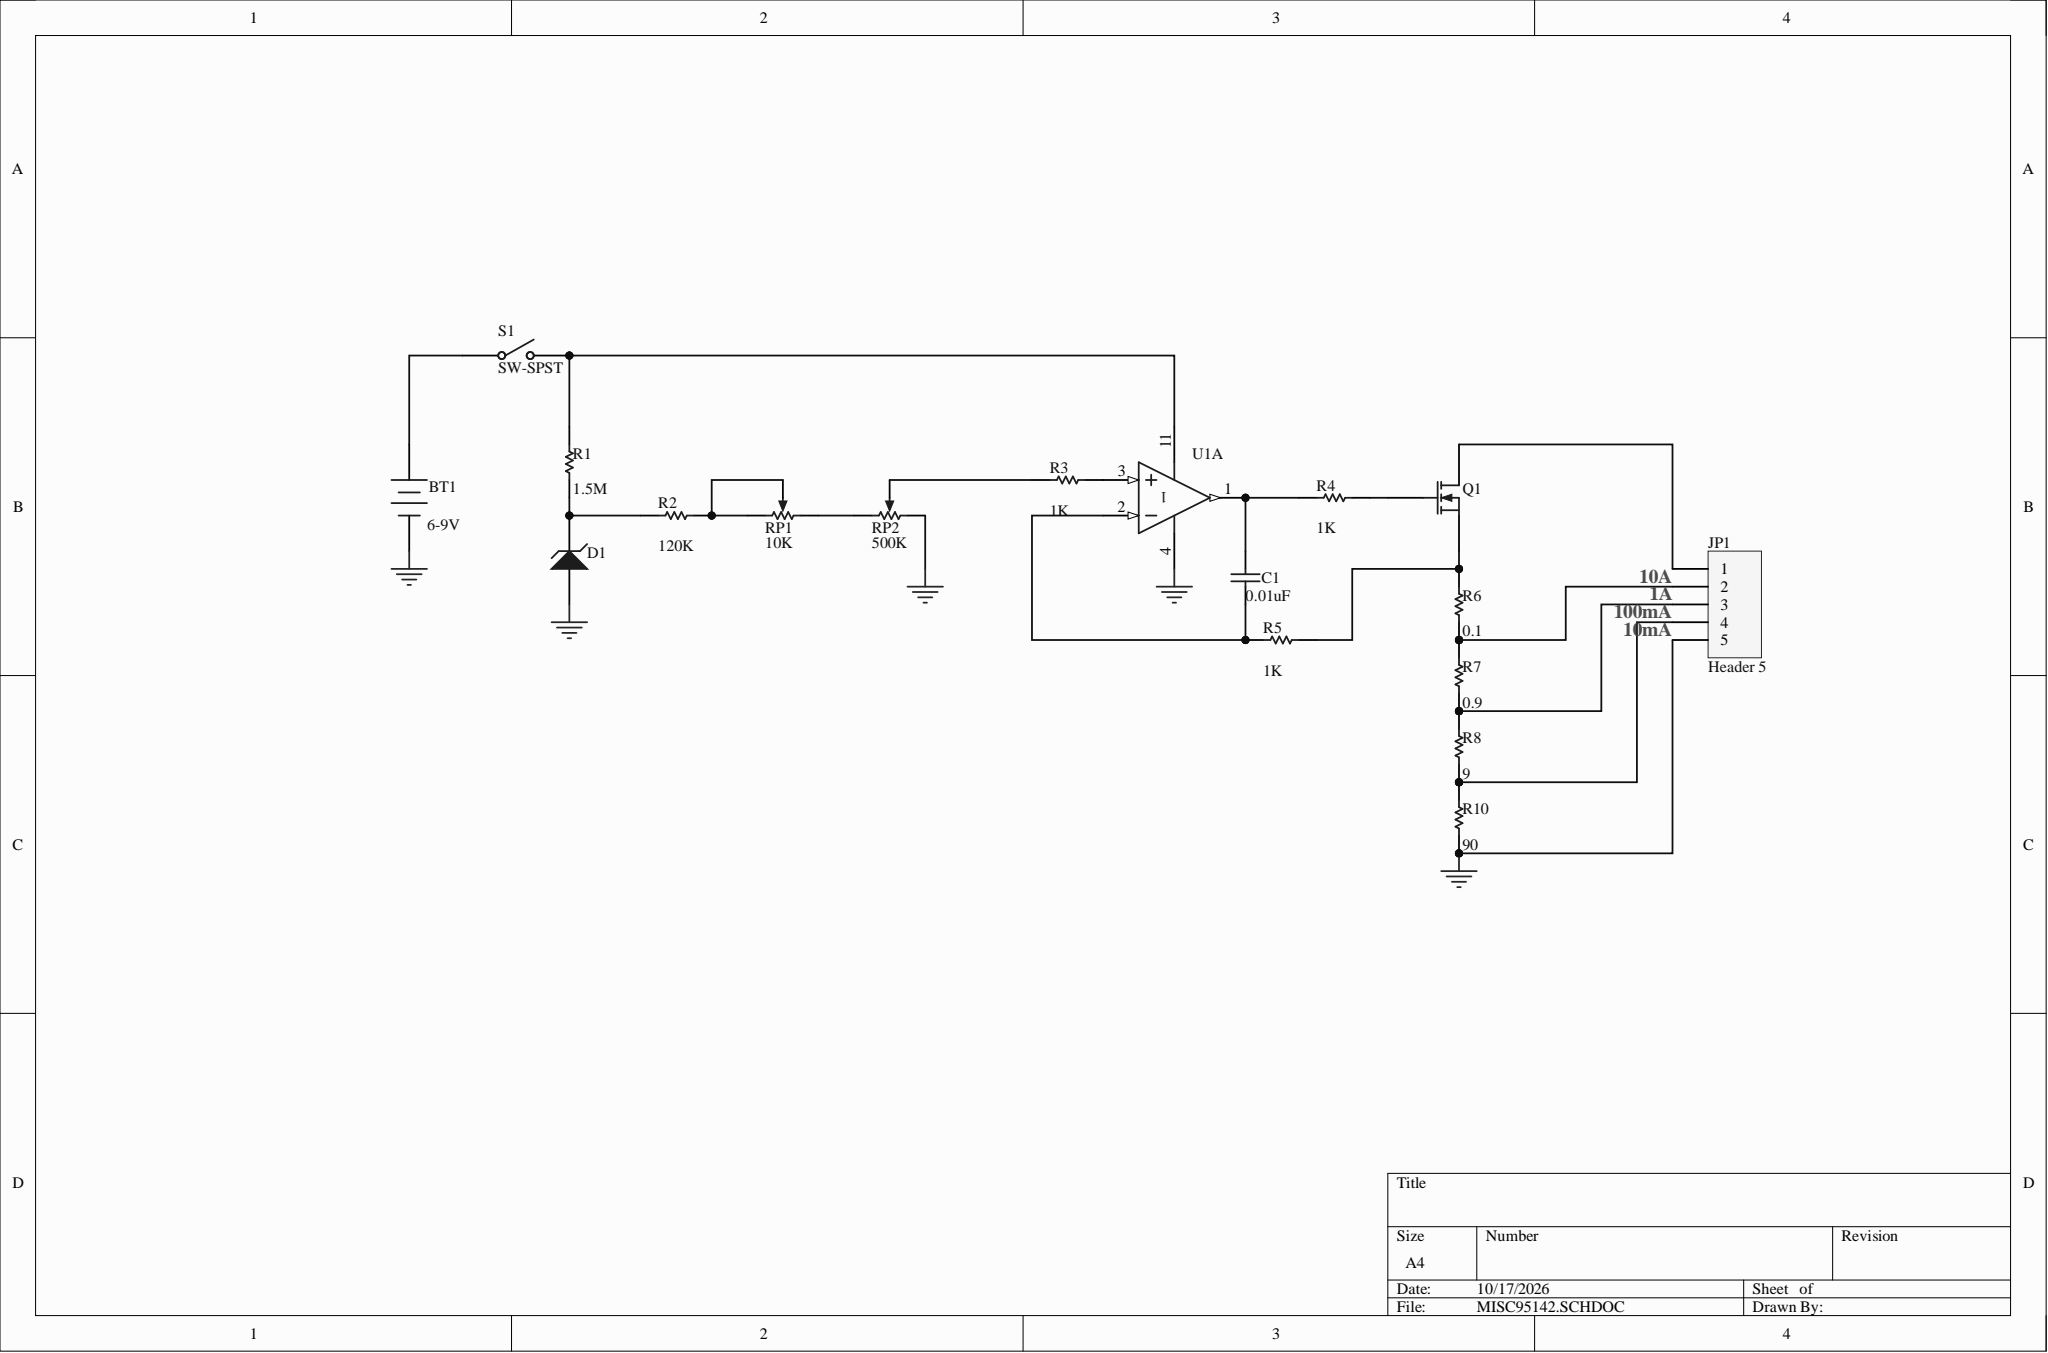Circuit board | Altium Designer | 18 parts | 16 nets
Bill of materials:
Comment,Description,Designator,Footprint,LibRef,Quantity
"Battery","Multicell Battery","BT1","BAT-2","Battery","1"
"Cap","Capacitor","C1","RAD-0.3","Cap","1"
"D Zener","Zener Diode","D1","DIODE-0.7","D Zener","1"
"Header 5","Header, 5-Pin","JP1","HDR1X5","Header 5","1"
"MOSFET-N","N-Channel MOSFET","Q1","BCY-W3/H.8","MOSFET-N","1"
"Res1","Resistor","R1, R2, R3, R4, R5, R6, R7, R8, R10","AXIAL-0.3","Res1","9"
"RPot","Potentiometer","RP1, RP2","VR2","RPot","2"
"SW-SPST","Single-Pole, Single-Throw Switch","S1","SPST-2","SW-SPST","1"
"LM248J","Quadruple Operational Amplifier","U1","J014","LM248J","1"
Netlist (Protel format):
[
BT1
BAT-2
Battery



]
[
C1
RAD-0.3
Cap



]
[
D1
DIODE-0.7
D Zener



]
[
JP1
HDR1X5
Header 5



]
[
Q1
BCY-W3/H.8
MOSFET-N



]
[
R1
AXIAL-0.3
Res1



]
[
R2
AXIAL-0.3
Res1



]
[
R3
AXIAL-0.3
Res1



]
[
R4
AXIAL-0.3
Res1



]
[
R5
AXIAL-0.3
Res1



]
[
R6
AXIAL-0.3
Res1



]
[
R7
AXIAL-0.3
Res1



]
[
R8
AXIAL-0.3
Res1



]
[
R10
AXIAL-0.3
Res1



]
[
RP1
VR2
RPot



]
[
RP2
VR2
RPot



]
[
S1
SPST-2
SW-SPST



]
[
U1
J014
LM248J



]
(
NetRP1_1
RP1-1
RP2-2
)
(
NetR3_2
R3-2
U1-3
)
(
NetR3_1
R3-1
RP2-3
)
(
NetR2_2
R2-2
RP1-2
RP1-3
)
(
NetR1_2
R1-2
S1-2
U1-11
)
(
NetQ1_3
Q1-3
R5-2
R6-2
)
(
NetQ1_2
Q1-2
R4-2
)
(
NetJP1_4
JP1-4
R8-1
R10-2
)
(
NetJP1_3
JP1-3
R7-1
R8-2
)
(
NetJP1_2
JP1-2
R6-1
R7-2
)
(
NetJP1_1
JP1-1
Q1-1
)
(
NetD1_2
D1-2
R1-1
R2-1
)
(
NetC1_2
C1-2
R4-1
U1-1
)
(
NetC1_1
C1-1
R5-1
U1-2
)
(
NetBT1_1
BT1-1
S1-1
)
(
GND
BT1-2
D1-1
JP1-5
R10-1
RP2-1
U1-4
)